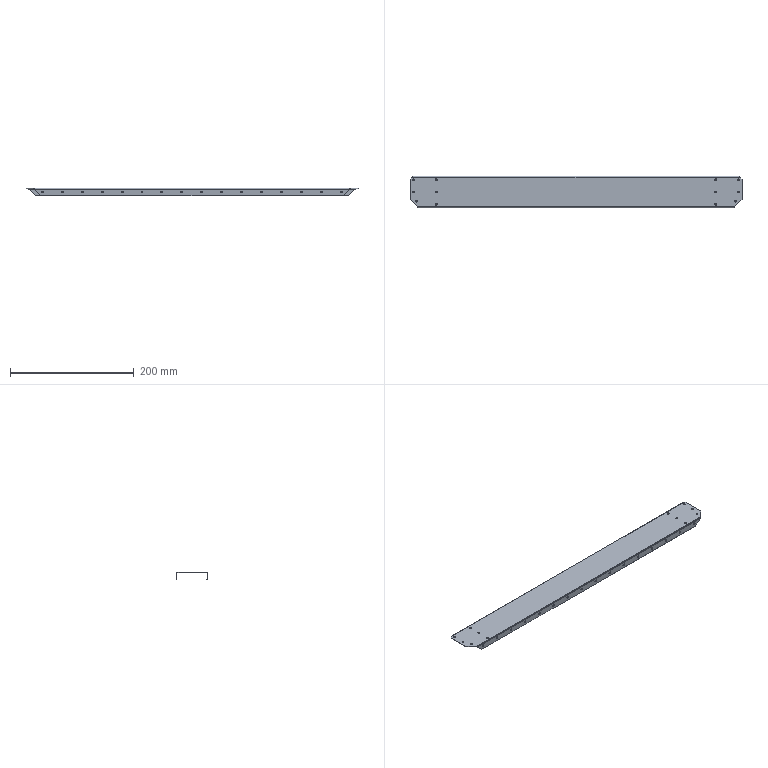Part | SolidWorks | features BaseBody 1 | 1 solid | 82 faces | box 536.6 x 50.892 x 11.991 mm | volume 19065 mm3 | cylinder 60 | plane 18 | spline 4 | commonest cylinder face diameters 3.2 x56 1.5 x2 2.5 x2